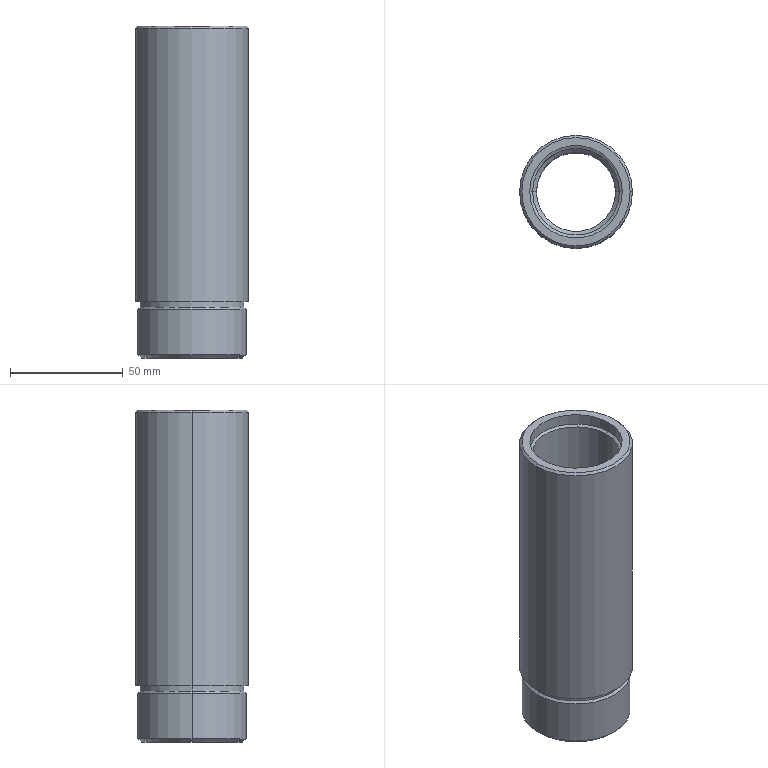Part | SolidWorks | features Chamfer 4, RevCut 2, Extrusion 1, ICE 1 | 1 solid | 25 faces | box 50 x 50 x 147 mm | volume 134333 mm3 | cylinder 12 | cone 10 | plane 3 | commonest cylinder face diameters 35 x2 38.5 x2 41 x2 46 x2 48 x2 50 x2
STEP:
#1=CARTESIAN_POINT('',(-17.5,0.,109.));
#2=VERTEX_POINT('',#1);
#3=CARTESIAN_POINT('',(17.5,0.,109.));
#4=VERTEX_POINT('',#3);
#5=CARTESIAN_POINT('',(0.,0.,109.));
#6=DIRECTION('',(0.,0.,1.));
#7=DIRECTION('',(1.,0.,0.));
#8=AXIS2_PLACEMENT_3D('',#5,#6,#7);
#9=CIRCLE('',#8,17.5);
#10=EDGE_CURVE('',#2,#4,#9,.T.);
#11=ORIENTED_EDGE('',*,*,#10,.F.);
#12=CARTESIAN_POINT('',(-19.25,0.,110.75));
#13=VERTEX_POINT('',#12);
#14=CARTESIAN_POINT('',(-19.25,0.,110.75));
#15=DIRECTION('',(-0.7071,0.,0.7071));
#16=VECTOR('',#15,1000.);
#17=LINE('',#14,#16);
#18=EDGE_CURVE('',#2,#13,#17,.T.);
#19=ORIENTED_EDGE('',*,*,#18,.T.);
#20=CARTESIAN_POINT('',(19.25,0.,110.75));
#21=VERTEX_POINT('',#20);
#22=CARTESIAN_POINT('',(0.,0.,110.75));
#23=DIRECTION('',(0.,0.,-1.));
#24=DIRECTION('',(1.,0.,0.));
#25=AXIS2_PLACEMENT_3D('',#22,#23,#24);
#26=CIRCLE('',#25,19.25);
#27=EDGE_CURVE('',#21,#13,#26,.T.);
#28=ORIENTED_EDGE('',*,*,#27,.F.);
#29=CARTESIAN_POINT('',(19.25,0.,110.75));
#30=DIRECTION('',(0.7071,0.,0.7071));
#31=VECTOR('',#30,1000.);
#32=LINE('',#29,#31);
#33=EDGE_CURVE('',#4,#21,#32,.T.);
#34=ORIENTED_EDGE('',*,*,#33,.F.);
#35=EDGE_LOOP('',(#11,#19,#28,#34));
#36=FACE_OUTER_BOUND('',#35,.T.);
#37=CARTESIAN_POINT('',(0.,0.,110.75));
#38=DIRECTION('',(0.,0.,1.));
#39=DIRECTION('',(1.,0.,0.));
#40=AXIS2_PLACEMENT_3D('',#37,#38,#39);
#41=CONICAL_SURFACE('',#40,19.25,0.7854);
#42=ADVANCED_FACE('',(#36),#41,.F.);
#43=CARTESIAN_POINT('',(19.25,0.,141.278));
#44=VERTEX_POINT('',#43);
#45=CARTESIAN_POINT('',(-19.25,0.,141.278));
#46=VERTEX_POINT('',#45);
#47=CARTESIAN_POINT('',(0.,0.,141.278));
#48=DIRECTION('',(0.,0.,-1.));
#49=DIRECTION('',(-1.,0.,0.));
#50=AXIS2_PLACEMENT_3D('',#47,#48,#49);
#51=CIRCLE('',#50,19.25);
#52=EDGE_CURVE('',#44,#46,#51,.T.);
#53=ORIENTED_EDGE('',*,*,#52,.F.);
#54=CARTESIAN_POINT('',(19.25,0.,0.));
#55=DIRECTION('',(0.,0.,-1.));
#56=VECTOR('',#55,1000.);
#57=LINE('',#54,#56);
#58=EDGE_CURVE('',#44,#21,#57,.T.);
#59=ORIENTED_EDGE('',*,*,#58,.T.);
#60=ORIENTED_EDGE('',*,*,#27,.T.);
#61=CARTESIAN_POINT('',(-19.25,0.,0.));
#62=DIRECTION('',(0.,0.,-1.));
#63=VECTOR('',#62,1000.);
#64=LINE('',#61,#63);
#65=EDGE_CURVE('',#46,#13,#64,.T.);
#66=ORIENTED_EDGE('',*,*,#65,.F.);
#67=EDGE_LOOP('',(#53,#59,#60,#66));
#68=FACE_OUTER_BOUND('',#67,.T.);
#69=CARTESIAN_POINT('',(0.,0.,0.));
#70=DIRECTION('',(0.,0.,-1.));
#71=DIRECTION('',(-1.,0.,0.));
#72=AXIS2_PLACEMENT_3D('',#69,#70,#71);
#73=CYLINDRICAL_SURFACE('',#72,19.25);
#74=ADVANCED_FACE('',(#68),#73,.F.);
#75=ORIENTED_EDGE('',*,*,#52,.T.);
#76=CARTESIAN_POINT('',(-20.5,0.,142.));
#77=VERTEX_POINT('',#76);
#78=CARTESIAN_POINT('',(-20.5,0.,142.));
#79=DIRECTION('',(-0.866,0.,0.5));
#80=VECTOR('',#79,1000.);
#81=LINE('',#78,#80);
#82=EDGE_CURVE('',#46,#77,#81,.T.);
#83=ORIENTED_EDGE('',*,*,#82,.T.);
#84=CARTESIAN_POINT('',(20.5,0.,142.));
#85=VERTEX_POINT('',#84);
#86=CARTESIAN_POINT('',(0.,0.,142.));
#87=DIRECTION('',(0.,0.,-1.));
#88=DIRECTION('',(-1.,0.,0.));
#89=AXIS2_PLACEMENT_3D('',#86,#87,#88);
#90=CIRCLE('',#89,20.5);
#91=EDGE_CURVE('',#85,#77,#90,.T.);
#92=ORIENTED_EDGE('',*,*,#91,.F.);
#93=CARTESIAN_POINT('',(20.5,0.,142.));
#94=DIRECTION('',(0.866,0.,0.5));
#95=VECTOR('',#94,1000.);
#96=LINE('',#93,#95);
#97=EDGE_CURVE('',#44,#85,#96,.T.);
#98=ORIENTED_EDGE('',*,*,#97,.F.);
#99=EDGE_LOOP('',(#75,#83,#92,#98));
#100=FACE_OUTER_BOUND('',#99,.T.);
#101=CARTESIAN_POINT('',(0.,0.,142.));
#102=DIRECTION('',(0.,0.,1.));
#103=DIRECTION('',(1.,0.,0.));
#104=AXIS2_PLACEMENT_3D('',#101,#102,#103);
#105=CONICAL_SURFACE('',#104,20.5,1.047);
#106=ADVANCED_FACE('',(#100),#105,.F.);
#107=CARTESIAN_POINT('',(20.5,0.,147.));
#108=VERTEX_POINT('',#107);
#109=CARTESIAN_POINT('',(-20.5,0.,147.));
#110=VERTEX_POINT('',#109);
#111=CARTESIAN_POINT('',(0.,0.,147.));
#112=DIRECTION('',(0.,0.,-1.));
#113=DIRECTION('',(-1.,0.,0.));
#114=AXIS2_PLACEMENT_3D('',#111,#112,#113);
#115=CIRCLE('',#114,20.5);
#116=EDGE_CURVE('',#108,#110,#115,.T.);
#117=ORIENTED_EDGE('',*,*,#116,.F.);
#118=CARTESIAN_POINT('',(20.5,0.,0.));
#119=DIRECTION('',(0.,0.,-1.));
#120=VECTOR('',#119,1000.);
#121=LINE('',#118,#120);
#122=EDGE_CURVE('',#108,#85,#121,.T.);
#123=ORIENTED_EDGE('',*,*,#122,.T.);
#124=ORIENTED_EDGE('',*,*,#91,.T.);
#125=CARTESIAN_POINT('',(-20.5,0.,0.));
#126=DIRECTION('',(0.,0.,-1.));
#127=VECTOR('',#126,1000.);
#128=LINE('',#125,#127);
#129=EDGE_CURVE('',#110,#77,#128,.T.);
#130=ORIENTED_EDGE('',*,*,#129,.F.);
#131=EDGE_LOOP('',(#117,#123,#124,#130));
#132=FACE_OUTER_BOUND('',#131,.T.);
#133=CARTESIAN_POINT('',(0.,0.,0.));
#134=DIRECTION('',(0.,0.,-1.));
#135=DIRECTION('',(-1.,0.,0.));
#136=AXIS2_PLACEMENT_3D('',#133,#134,#135);
#137=CYLINDRICAL_SURFACE('',#136,20.5);
#138=ADVANCED_FACE('',(#132),#137,.F.);
#139=CARTESIAN_POINT('',(24.,0.,147.));
#140=VERTEX_POINT('',#139);
#141=CARTESIAN_POINT('',(-24.,0.,147.));
#142=VERTEX_POINT('',#141);
#143=CARTESIAN_POINT('',(0.,0.,147.));
#144=DIRECTION('',(0.,0.,1.));
#145=DIRECTION('',(1.,0.,0.));
#146=AXIS2_PLACEMENT_3D('',#143,#144,#145);
#147=CIRCLE('',#146,24.);
#148=EDGE_CURVE('',#140,#142,#147,.T.);
#149=ORIENTED_EDGE('',*,*,#148,.F.);
#150=CARTESIAN_POINT('',(25.,0.,146.));
#151=VERTEX_POINT('',#150);
#152=CARTESIAN_POINT('',(24.,0.,147.));
#153=DIRECTION('',(0.7071,0.,-0.7071));
#154=VECTOR('',#153,1000.);
#155=LINE('',#152,#154);
#156=EDGE_CURVE('',#140,#151,#155,.T.);
#157=ORIENTED_EDGE('',*,*,#156,.T.);
#158=CARTESIAN_POINT('',(-25.,0.,146.));
#159=VERTEX_POINT('',#158);
#160=CARTESIAN_POINT('',(0.,0.,146.));
#161=DIRECTION('',(0.,0.,-1.));
#162=DIRECTION('',(1.,0.,0.));
#163=AXIS2_PLACEMENT_3D('',#160,#161,#162);
#164=CIRCLE('',#163,25.);
#165=EDGE_CURVE('',#159,#151,#164,.T.);
#166=ORIENTED_EDGE('',*,*,#165,.F.);
#167=CARTESIAN_POINT('',(-24.,0.,147.));
#168=DIRECTION('',(-0.7071,0.,-0.7071));
#169=VECTOR('',#168,1000.);
#170=LINE('',#167,#169);
#171=EDGE_CURVE('',#142,#159,#170,.T.);
#172=ORIENTED_EDGE('',*,*,#171,.F.);
#173=EDGE_LOOP('',(#149,#157,#166,#172));
#174=FACE_OUTER_BOUND('',#173,.T.);
#175=CARTESIAN_POINT('',(0.,0.,147.));
#176=DIRECTION('',(0.,0.,-1.));
#177=DIRECTION('',(-1.,0.,0.));
#178=AXIS2_PLACEMENT_3D('',#175,#176,#177);
#179=CONICAL_SURFACE('',#178,24.,0.7854);
#180=ADVANCED_FACE('',(#174),#179,.T.);
#181=CARTESIAN_POINT('',(-22.5,0.,0.));
#182=VERTEX_POINT('',#181);
#183=CARTESIAN_POINT('',(22.5,0.,0.));
#184=VERTEX_POINT('',#183);
#185=CARTESIAN_POINT('',(0.,0.,0.));
#186=DIRECTION('',(0.,0.,-1.));
#187=DIRECTION('',(1.,0.,0.));
#188=AXIS2_PLACEMENT_3D('',#185,#186,#187);
#189=CIRCLE('',#188,22.5);
#190=EDGE_CURVE('',#182,#184,#189,.T.);
#191=ORIENTED_EDGE('',*,*,#190,.F.);
#192=CARTESIAN_POINT('',(-24.,0.,1.5));
#193=VERTEX_POINT('',#192);
#194=CARTESIAN_POINT('',(-22.5,0.,0.));
#195=DIRECTION('',(-0.7071,0.,0.7071));
#196=VECTOR('',#195,1000.);
#197=LINE('',#194,#196);
#198=EDGE_CURVE('',#182,#193,#197,.T.);
#199=ORIENTED_EDGE('',*,*,#198,.T.);
#200=CARTESIAN_POINT('',(24.,0.,1.5));
#201=VERTEX_POINT('',#200);
#202=CARTESIAN_POINT('',(0.,0.,1.5));
#203=DIRECTION('',(0.,0.,1.));
#204=DIRECTION('',(1.,0.,0.));
#205=AXIS2_PLACEMENT_3D('',#202,#203,#204);
#206=CIRCLE('',#205,24.);
#207=EDGE_CURVE('',#201,#193,#206,.T.);
#208=ORIENTED_EDGE('',*,*,#207,.F.);
#209=CARTESIAN_POINT('',(22.5,0.,0.));
#210=DIRECTION('',(0.7071,0.,0.7071));
#211=VECTOR('',#210,1000.);
#212=LINE('',#209,#211);
#213=EDGE_CURVE('',#184,#201,#212,.T.);
#214=ORIENTED_EDGE('',*,*,#213,.F.);
#215=EDGE_LOOP('',(#191,#199,#208,#214));
#216=FACE_OUTER_BOUND('',#215,.T.);
#217=CARTESIAN_POINT('',(0.,0.,0.));
#218=DIRECTION('',(0.,0.,1.));
#219=DIRECTION('',(1.,0.,0.));
#220=AXIS2_PLACEMENT_3D('',#217,#218,#219);
#221=CONICAL_SURFACE('',#220,22.5,0.7854);
#222=ADVANCED_FACE('',(#216),#221,.T.);
#223=CARTESIAN_POINT('',(23.,0.,22.5));
#224=VERTEX_POINT('',#223);
#225=CARTESIAN_POINT('',(-23.,0.,22.5));
#226=VERTEX_POINT('',#225);
#227=CARTESIAN_POINT('',(0.,0.,22.5));
#228=DIRECTION('',(0.,0.,1.));
#229=DIRECTION('',(-1.,0.,0.));
#230=AXIS2_PLACEMENT_3D('',#227,#228,#229);
#231=CIRCLE('',#230,23.);
#232=EDGE_CURVE('',#224,#226,#231,.T.);
#233=ORIENTED_EDGE('',*,*,#232,.F.);
#234=CARTESIAN_POINT('',(24.,0.,21.5));
#235=VERTEX_POINT('',#234);
#236=CARTESIAN_POINT('',(24.,0.,21.5));
#237=DIRECTION('',(0.7071,0.,-0.7071));
#238=VECTOR('',#237,1000.);
#239=LINE('',#236,#238);
#240=EDGE_CURVE('',#224,#235,#239,.T.);
#241=ORIENTED_EDGE('',*,*,#240,.T.);
#242=CARTESIAN_POINT('',(-24.,0.,21.5));
#243=VERTEX_POINT('',#242);
#244=CARTESIAN_POINT('',(0.,0.,21.5));
#245=DIRECTION('',(0.,0.,-1.));
#246=DIRECTION('',(1.,0.,0.));
#247=AXIS2_PLACEMENT_3D('',#244,#245,#246);
#248=CIRCLE('',#247,24.);
#249=EDGE_CURVE('',#243,#235,#248,.T.);
#250=ORIENTED_EDGE('',*,*,#249,.F.);
#251=CARTESIAN_POINT('',(-24.,0.,21.5));
#252=DIRECTION('',(-0.7071,0.,-0.7071));
#253=VECTOR('',#252,1000.);
#254=LINE('',#251,#253);
#255=EDGE_CURVE('',#226,#243,#254,.T.);
#256=ORIENTED_EDGE('',*,*,#255,.F.);
#257=EDGE_LOOP('',(#233,#241,#250,#256));
#258=FACE_OUTER_BOUND('',#257,.T.);
#259=CARTESIAN_POINT('',(0.,0.,21.5));
#260=DIRECTION('',(0.,0.,-1.));
#261=DIRECTION('',(-1.,0.,0.));
#262=AXIS2_PLACEMENT_3D('',#259,#260,#261);
#263=CONICAL_SURFACE('',#262,24.,0.7854);
#264=ADVANCED_FACE('',(#258),#263,.T.);
#265=CARTESIAN_POINT('',(-23.,0.,25.));
#266=VERTEX_POINT('',#265);
#267=CARTESIAN_POINT('',(23.,0.,25.));
#268=VERTEX_POINT('',#267);
#269=CARTESIAN_POINT('',(0.,0.,25.));
#270=DIRECTION('',(0.,0.,-1.));
#271=DIRECTION('',(-1.,0.,0.));
#272=AXIS2_PLACEMENT_3D('',#269,#270,#271);
#273=CIRCLE('',#272,23.);
#274=EDGE_CURVE('',#266,#268,#273,.T.);
#275=ORIENTED_EDGE('',*,*,#274,.T.);
#276=CARTESIAN_POINT('',(23.,0.,0.));
#277=DIRECTION('',(0.,0.,-1.));
#278=VECTOR('',#277,1000.);
#279=LINE('',#276,#278);
#280=EDGE_CURVE('',#268,#224,#279,.T.);
#281=ORIENTED_EDGE('',*,*,#280,.T.);
#282=ORIENTED_EDGE('',*,*,#232,.T.);
#283=CARTESIAN_POINT('',(-23.,0.,0.));
#284=DIRECTION('',(0.,0.,-1.));
#285=VECTOR('',#284,1000.);
#286=LINE('',#283,#285);
#287=EDGE_CURVE('',#266,#226,#286,.T.);
#288=ORIENTED_EDGE('',*,*,#287,.F.);
#289=EDGE_LOOP('',(#275,#281,#282,#288));
#290=FACE_OUTER_BOUND('',#289,.T.);
#291=CARTESIAN_POINT('',(0.,0.,0.));
#292=DIRECTION('',(0.,0.,-1.));
#293=DIRECTION('',(-1.,0.,0.));
#294=AXIS2_PLACEMENT_3D('',#291,#292,#293);
#295=CYLINDRICAL_SURFACE('',#294,23.);
#296=ADVANCED_FACE('',(#290),#295,.T.);
#297=ORIENTED_EDGE('',*,*,#249,.T.);
#298=CARTESIAN_POINT('',(24.,0.,0.));
#299=DIRECTION('',(0.,0.,-1.));
#300=VECTOR('',#299,1000.);
#301=LINE('',#298,#300);
#302=EDGE_CURVE('',#235,#201,#301,.T.);
#303=ORIENTED_EDGE('',*,*,#302,.T.);
#304=ORIENTED_EDGE('',*,*,#207,.T.);
#305=CARTESIAN_POINT('',(-24.,0.,0.));
#306=DIRECTION('',(0.,0.,-1.));
#307=VECTOR('',#306,1000.);
#308=LINE('',#305,#307);
#309=EDGE_CURVE('',#243,#193,#308,.T.);
#310=ORIENTED_EDGE('',*,*,#309,.F.);
#311=EDGE_LOOP('',(#297,#303,#304,#310));
#312=FACE_OUTER_BOUND('',#311,.T.);
#313=CARTESIAN_POINT('',(0.,0.,0.));
#314=DIRECTION('',(0.,0.,-1.));
#315=DIRECTION('',(-1.,0.,0.));
#316=AXIS2_PLACEMENT_3D('',#313,#314,#315);
#317=CYLINDRICAL_SURFACE('',#316,24.);
#318=ADVANCED_FACE('',(#312),#317,.T.);
#319=ORIENTED_EDGE('',*,*,#165,.T.);
#320=CARTESIAN_POINT('',(25.,0.,25.));
#321=VERTEX_POINT('',#320);
#322=CARTESIAN_POINT('',(25.,0.,147.));
#323=DIRECTION('',(0.,0.,-1.));
#324=VECTOR('',#323,1000.);
#325=LINE('',#322,#324);
#326=EDGE_CURVE('',#151,#321,#325,.T.);
#327=ORIENTED_EDGE('',*,*,#326,.T.);
#328=CARTESIAN_POINT('',(-25.,0.,25.));
#329=VERTEX_POINT('',#328);
#330=CARTESIAN_POINT('',(0.,0.,25.));
#331=DIRECTION('',(0.,0.,-1.));
#332=DIRECTION('',(-1.,0.,0.));
#333=AXIS2_PLACEMENT_3D('',#330,#331,#332);
#334=CIRCLE('',#333,25.);
#335=EDGE_CURVE('',#329,#321,#334,.T.);
#336=ORIENTED_EDGE('',*,*,#335,.F.);
#337=CARTESIAN_POINT('',(-25.,0.,147.));
#338=DIRECTION('',(0.,0.,-1.));
#339=VECTOR('',#338,1000.);
#340=LINE('',#337,#339);
#341=EDGE_CURVE('',#159,#329,#340,.T.);
#342=ORIENTED_EDGE('',*,*,#341,.F.);
#343=EDGE_LOOP('',(#319,#327,#336,#342));
#344=FACE_OUTER_BOUND('',#343,.T.);
#345=CARTESIAN_POINT('',(0.,0.,147.));
#346=DIRECTION('',(0.,0.,-1.));
#347=DIRECTION('',(-1.,0.,0.));
#348=AXIS2_PLACEMENT_3D('',#345,#346,#347);
#349=CYLINDRICAL_SURFACE('',#348,25.);
#350=ADVANCED_FACE('',(#344),#349,.T.);
#351=ORIENTED_EDGE('',*,*,#10,.T.);
#352=CARTESIAN_POINT('',(17.5,0.,0.));
#353=VERTEX_POINT('',#352);
#354=CARTESIAN_POINT('',(17.5,0.,147.));
#355=DIRECTION('',(0.,0.,-1.));
#356=VECTOR('',#355,1000.);
#357=LINE('',#354,#356);
#358=EDGE_CURVE('',#4,#353,#357,.T.);
#359=ORIENTED_EDGE('',*,*,#358,.T.);
#360=CARTESIAN_POINT('',(-17.5,0.,0.));
#361=VERTEX_POINT('',#360);
#362=CARTESIAN_POINT('',(0.,0.,0.));
#363=DIRECTION('',(0.,0.,1.));
#364=DIRECTION('',(1.,0.,0.));
#365=AXIS2_PLACEMENT_3D('',#362,#363,#364);
#366=CIRCLE('',#365,17.5);
#367=EDGE_CURVE('',#361,#353,#366,.T.);
#368=ORIENTED_EDGE('',*,*,#367,.F.);
#369=CARTESIAN_POINT('',(-17.5,0.,147.));
#370=DIRECTION('',(0.,0.,-1.));
#371=VECTOR('',#370,1000.);
#372=LINE('',#369,#371);
#373=EDGE_CURVE('',#2,#361,#372,.T.);
#374=ORIENTED_EDGE('',*,*,#373,.F.);
#375=EDGE_LOOP('',(#351,#359,#368,#374));
#376=FACE_OUTER_BOUND('',#375,.T.);
#377=CARTESIAN_POINT('',(0.,0.,147.));
#378=DIRECTION('',(0.,0.,-1.));
#379=DIRECTION('',(-1.,0.,0.));
#380=AXIS2_PLACEMENT_3D('',#377,#378,#379);
#381=CYLINDRICAL_SURFACE('',#380,17.5);
#382=ADVANCED_FACE('',(#376),#381,.F.);
#383=ORIENTED_EDGE('',*,*,#358,.F.);
#384=CARTESIAN_POINT('',(0.,0.,109.));
#385=DIRECTION('',(0.,0.,1.));
#386=DIRECTION('',(1.,0.,0.));
#387=AXIS2_PLACEMENT_3D('',#384,#385,#386);
#388=CIRCLE('',#387,17.5);
#389=EDGE_CURVE('',#4,#2,#388,.T.);
#390=ORIENTED_EDGE('',*,*,#389,.T.);
#391=ORIENTED_EDGE('',*,*,#373,.T.);
#392=CARTESIAN_POINT('',(0.,0.,0.));
#393=DIRECTION('',(0.,0.,1.));
#394=DIRECTION('',(1.,0.,0.));
#395=AXIS2_PLACEMENT_3D('',#392,#393,#394);
#396=CIRCLE('',#395,17.5);
#397=EDGE_CURVE('',#353,#361,#396,.T.);
#398=ORIENTED_EDGE('',*,*,#397,.F.);
#399=EDGE_LOOP('',(#383,#390,#391,#398));
#400=FACE_OUTER_BOUND('',#399,.T.);
#401=CARTESIAN_POINT('',(0.,0.,147.));
#402=DIRECTION('',(0.,0.,-1.));
#403=DIRECTION('',(-1.,0.,0.));
#404=AXIS2_PLACEMENT_3D('',#401,#402,#403);
#405=CYLINDRICAL_SURFACE('',#404,17.5);
#406=ADVANCED_FACE('',(#400),#405,.F.);
#407=CARTESIAN_POINT('',(0.,0.,0.));
#408=DIRECTION('',(0.,0.,-1.));
#409=DIRECTION('',(1.,0.,0.));
#410=AXIS2_PLACEMENT_3D('',#407,#408,#409);
#411=CIRCLE('',#410,22.5);
#412=EDGE_CURVE('',#184,#182,#411,.T.);
#413=ORIENTED_EDGE('',*,*,#412,.T.);
#414=ORIENTED_EDGE('',*,*,#190,.T.);
#415=EDGE_LOOP('',(#413,#414));
#416=FACE_OUTER_BOUND('',#415,.T.);
#417=ORIENTED_EDGE('',*,*,#367,.T.);
#418=ORIENTED_EDGE('',*,*,#397,.T.);
#419=EDGE_LOOP('',(#417,#418));
#420=FACE_BOUND('',#419,.T.);
#421=CARTESIAN_POINT('',(0.,0.,0.));
#422=DIRECTION('',(0.,0.,1.));
#423=DIRECTION('',(1.,0.,0.));
#424=AXIS2_PLACEMENT_3D('',#421,#422,#423);
#425=PLANE('',#424);
#426=ADVANCED_FACE('',(#416,#420),#425,.F.);
#427=ORIENTED_EDGE('',*,*,#326,.F.);
#428=CARTESIAN_POINT('',(0.,0.,146.));
#429=DIRECTION('',(0.,0.,-1.));
#430=DIRECTION('',(1.,0.,0.));
#431=AXIS2_PLACEMENT_3D('',#428,#429,#430);
#432=CIRCLE('',#431,25.);
#433=EDGE_CURVE('',#151,#159,#432,.T.);
#434=ORIENTED_EDGE('',*,*,#433,.T.);
#435=ORIENTED_EDGE('',*,*,#341,.T.);
#436=CARTESIAN_POINT('',(0.,0.,25.));
#437=DIRECTION('',(0.,0.,-1.));
#438=DIRECTION('',(-1.,0.,0.));
#439=AXIS2_PLACEMENT_3D('',#436,#437,#438);
#440=CIRCLE('',#439,25.);
#441=EDGE_CURVE('',#321,#329,#440,.T.);
#442=ORIENTED_EDGE('',*,*,#441,.F.);
#443=EDGE_LOOP('',(#427,#434,#435,#442));
#444=FACE_OUTER_BOUND('',#443,.T.);
#445=CARTESIAN_POINT('',(0.,0.,147.));
#446=DIRECTION('',(0.,0.,-1.));
#447=DIRECTION('',(-1.,0.,0.));
#448=AXIS2_PLACEMENT_3D('',#445,#446,#447);
#449=CYLINDRICAL_SURFACE('',#448,25.);
#450=ADVANCED_FACE('',(#444),#449,.T.);
#451=CARTESIAN_POINT('',(0.,0.,147.));
#452=DIRECTION('',(0.,0.,-1.));
#453=DIRECTION('',(-1.,0.,0.));
#454=AXIS2_PLACEMENT_3D('',#451,#452,#453);
#455=CIRCLE('',#454,20.5);
#456=EDGE_CURVE('',#110,#108,#455,.T.);
#457=ORIENTED_EDGE('',*,*,#456,.T.);
#458=ORIENTED_EDGE('',*,*,#116,.T.);
#459=EDGE_LOOP('',(#457,#458));
#460=FACE_BOUND('',#459,.T.);
#461=CARTESIAN_POINT('',(0.,0.,147.));
#462=DIRECTION('',(0.,0.,1.));
#463=DIRECTION('',(1.,0.,0.));
#464=AXIS2_PLACEMENT_3D('',#461,#462,#463);
#465=CIRCLE('',#464,24.);
#466=EDGE_CURVE('',#142,#140,#465,.T.);
#467=ORIENTED_EDGE('',*,*,#466,.T.);
#468=ORIENTED_EDGE('',*,*,#148,.T.);
#469=EDGE_LOOP('',(#467,#468));
#470=FACE_OUTER_BOUND('',#469,.T.);
#471=CARTESIAN_POINT('',(0.,0.,147.));
#472=DIRECTION('',(0.,0.,1.));
#473=DIRECTION('',(1.,0.,0.));
#474=AXIS2_PLACEMENT_3D('',#471,#472,#473);
#475=PLANE('',#474);
#476=ADVANCED_FACE('',(#460,#470),#475,.T.);
#477=ORIENTED_EDGE('',*,*,#302,.F.);
#478=CARTESIAN_POINT('',(0.,0.,21.5));
#479=DIRECTION('',(0.,0.,-1.));
#480=DIRECTION('',(1.,0.,0.));
#481=AXIS2_PLACEMENT_3D('',#478,#479,#480);
#482=CIRCLE('',#481,24.);
#483=EDGE_CURVE('',#235,#243,#482,.T.);
#484=ORIENTED_EDGE('',*,*,#483,.T.);
#485=ORIENTED_EDGE('',*,*,#309,.T.);
#486=CARTESIAN_POINT('',(0.,0.,1.5));
#487=DIRECTION('',(0.,0.,1.));
#488=DIRECTION('',(1.,0.,0.));
#489=AXIS2_PLACEMENT_3D('',#486,#487,#488);
#490=CIRCLE('',#489,24.);
#491=EDGE_CURVE('',#193,#201,#490,.T.);
#492=ORIENTED_EDGE('',*,*,#491,.T.);
#493=EDGE_LOOP('',(#477,#484,#485,#492));
#494=FACE_OUTER_BOUND('',#493,.T.);
#495=CARTESIAN_POINT('',(0.,0.,0.));
#496=DIRECTION('',(0.,0.,-1.));
#497=DIRECTION('',(-1.,0.,0.));
#498=AXIS2_PLACEMENT_3D('',#495,#496,#497);
#499=CYLINDRICAL_SURFACE('',#498,24.);
#500=ADVANCED_FACE('',(#494),#499,.T.);
#501=ORIENTED_EDGE('',*,*,#280,.F.);
#502=CARTESIAN_POINT('',(0.,0.,25.));
#503=DIRECTION('',(0.,0.,-1.));
#504=DIRECTION('',(-1.,0.,0.));
#505=AXIS2_PLACEMENT_3D('',#502,#503,#504);
#506=CIRCLE('',#505,23.);
#507=EDGE_CURVE('',#268,#266,#506,.T.);
#508=ORIENTED_EDGE('',*,*,#507,.T.);
#509=ORIENTED_EDGE('',*,*,#287,.T.);
#510=CARTESIAN_POINT('',(0.,0.,22.5));
#511=DIRECTION('',(0.,0.,1.));
#512=DIRECTION('',(-1.,0.,0.));
#513=AXIS2_PLACEMENT_3D('',#510,#511,#512);
#514=CIRCLE('',#513,23.);
#515=EDGE_CURVE('',#226,#224,#514,.T.);
#516=ORIENTED_EDGE('',*,*,#515,.T.);
#517=EDGE_LOOP('',(#501,#508,#509,#516));
#518=FACE_OUTER_BOUND('',#517,.T.);
#519=CARTESIAN_POINT('',(0.,0.,0.));
#520=DIRECTION('',(0.,0.,-1.));
#521=DIRECTION('',(-1.,0.,0.));
#522=AXIS2_PLACEMENT_3D('',#519,#520,#521);
#523=CYLINDRICAL_SURFACE('',#522,23.);
#524=ADVANCED_FACE('',(#518),#523,.T.);
#525=ORIENTED_EDGE('',*,*,#335,.T.);
#526=ORIENTED_EDGE('',*,*,#441,.T.);
#527=EDGE_LOOP('',(#525,#526));
#528=FACE_OUTER_BOUND('',#527,.T.);
#529=ORIENTED_EDGE('',*,*,#274,.F.);
#530=ORIENTED_EDGE('',*,*,#507,.F.);
#531=EDGE_LOOP('',(#529,#530));
#532=FACE_BOUND('',#531,.T.);
#533=CARTESIAN_POINT('',(23.,0.,25.));
#534=DIRECTION('',(0.,0.,-1.));
#535=DIRECTION('',(-1.,0.,0.));
#536=AXIS2_PLACEMENT_3D('',#533,#534,#535);
#537=PLANE('',#536);
#538=ADVANCED_FACE('',(#528,#532),#537,.T.);
#539=ORIENTED_EDGE('',*,*,#240,.F.);
#540=ORIENTED_EDGE('',*,*,#515,.F.);
#541=ORIENTED_EDGE('',*,*,#255,.T.);
#542=ORIENTED_EDGE('',*,*,#483,.F.);
#543=EDGE_LOOP('',(#539,#540,#541,#542));
#544=FACE_OUTER_BOUND('',#543,.T.);
#545=CARTESIAN_POINT('',(0.,0.,21.5));
#546=DIRECTION('',(0.,0.,-1.));
#547=DIRECTION('',(-1.,0.,0.));
#548=AXIS2_PLACEMENT_3D('',#545,#546,#547);
#549=CONICAL_SURFACE('',#548,24.,0.7854);
#550=ADVANCED_FACE('',(#544),#549,.T.);
#551=ORIENTED_EDGE('',*,*,#198,.F.);
#552=ORIENTED_EDGE('',*,*,#412,.F.);
#553=ORIENTED_EDGE('',*,*,#213,.T.);
#554=ORIENTED_EDGE('',*,*,#491,.F.);
#555=EDGE_LOOP('',(#551,#552,#553,#554));
#556=FACE_OUTER_BOUND('',#555,.T.);
#557=CARTESIAN_POINT('',(0.,0.,0.));
#558=DIRECTION('',(0.,0.,1.));
#559=DIRECTION('',(1.,0.,0.));
#560=AXIS2_PLACEMENT_3D('',#557,#558,#559);
#561=CONICAL_SURFACE('',#560,22.5,0.7854);
#562=ADVANCED_FACE('',(#556),#561,.T.);
#563=ORIENTED_EDGE('',*,*,#156,.F.);
#564=ORIENTED_EDGE('',*,*,#466,.F.);
#565=ORIENTED_EDGE('',*,*,#171,.T.);
#566=ORIENTED_EDGE('',*,*,#433,.F.);
#567=EDGE_LOOP('',(#563,#564,#565,#566));
#568=FACE_OUTER_BOUND('',#567,.T.);
#569=CARTESIAN_POINT('',(0.,0.,147.));
#570=DIRECTION('',(0.,0.,-1.));
#571=DIRECTION('',(-1.,0.,0.));
#572=AXIS2_PLACEMENT_3D('',#569,#570,#571);
#573=CONICAL_SURFACE('',#572,24.,0.7854);
#574=ADVANCED_FACE('',(#568),#573,.T.);
#575=ORIENTED_EDGE('',*,*,#122,.F.);
#576=ORIENTED_EDGE('',*,*,#456,.F.);
#577=ORIENTED_EDGE('',*,*,#129,.T.);
#578=CARTESIAN_POINT('',(0.,0.,142.));
#579=DIRECTION('',(0.,0.,-1.));
#580=DIRECTION('',(-1.,0.,0.));
#581=AXIS2_PLACEMENT_3D('',#578,#579,#580);
#582=CIRCLE('',#581,20.5);
#583=EDGE_CURVE('',#77,#85,#582,.T.);
#584=ORIENTED_EDGE('',*,*,#583,.T.);
#585=EDGE_LOOP('',(#575,#576,#577,#584));
#586=FACE_OUTER_BOUND('',#585,.T.);
#587=CARTESIAN_POINT('',(0.,0.,0.));
#588=DIRECTION('',(0.,0.,-1.));
#589=DIRECTION('',(-1.,0.,0.));
#590=AXIS2_PLACEMENT_3D('',#587,#588,#589);
#591=CYLINDRICAL_SURFACE('',#590,20.5);
#592=ADVANCED_FACE('',(#586),#591,.F.);
#593=ORIENTED_EDGE('',*,*,#82,.F.);
#594=CARTESIAN_POINT('',(0.,0.,141.278));
#595=DIRECTION('',(0.,0.,-1.));
#596=DIRECTION('',(-1.,0.,0.));
#597=AXIS2_PLACEMENT_3D('',#594,#595,#596);
#598=CIRCLE('',#597,19.25);
#599=EDGE_CURVE('',#46,#44,#598,.T.);
#600=ORIENTED_EDGE('',*,*,#599,.T.);
#601=ORIENTED_EDGE('',*,*,#97,.T.);
#602=ORIENTED_EDGE('',*,*,#583,.F.);
#603=EDGE_LOOP('',(#593,#600,#601,#602));
#604=FACE_OUTER_BOUND('',#603,.T.);
#605=CARTESIAN_POINT('',(0.,0.,142.));
#606=DIRECTION('',(0.,0.,1.));
#607=DIRECTION('',(1.,0.,0.));
#608=AXIS2_PLACEMENT_3D('',#605,#606,#607);
#609=CONICAL_SURFACE('',#608,20.5,1.047);
#610=ADVANCED_FACE('',(#604),#609,.F.);
#611=ORIENTED_EDGE('',*,*,#58,.F.);
#612=ORIENTED_EDGE('',*,*,#599,.F.);
#613=ORIENTED_EDGE('',*,*,#65,.T.);
#614=CARTESIAN_POINT('',(0.,0.,110.75));
#615=DIRECTION('',(0.,0.,-1.));
#616=DIRECTION('',(1.,0.,0.));
#617=AXIS2_PLACEMENT_3D('',#614,#615,#616);
#618=CIRCLE('',#617,19.25);
#619=EDGE_CURVE('',#13,#21,#618,.T.);
#620=ORIENTED_EDGE('',*,*,#619,.T.);
#621=EDGE_LOOP('',(#611,#612,#613,#620));
#622=FACE_OUTER_BOUND('',#621,.T.);
#623=CARTESIAN_POINT('',(0.,0.,0.));
#624=DIRECTION('',(0.,0.,-1.));
#625=DIRECTION('',(-1.,0.,0.));
#626=AXIS2_PLACEMENT_3D('',#623,#624,#625);
#627=CYLINDRICAL_SURFACE('',#626,19.25);
#628=ADVANCED_FACE('',(#622),#627,.F.);
#629=ORIENTED_EDGE('',*,*,#18,.F.);
#630=ORIENTED_EDGE('',*,*,#389,.F.);
#631=ORIENTED_EDGE('',*,*,#33,.T.);
#632=ORIENTED_EDGE('',*,*,#619,.F.);
#633=EDGE_LOOP('',(#629,#630,#631,#632));
#634=FACE_OUTER_BOUND('',#633,.T.);
#635=CARTESIAN_POINT('',(0.,0.,110.75));
#636=DIRECTION('',(0.,0.,1.));
#637=DIRECTION('',(1.,0.,0.));
#638=AXIS2_PLACEMENT_3D('',#635,#636,#637);
#639=CONICAL_SURFACE('',#638,19.25,0.7854);
#640=ADVANCED_FACE('',(#634),#639,.F.);
#641=CLOSED_SHELL('',(#42,#74,#106,#138,#180,#222,#264,#296,#318,#350,#382,#406,#426,#450,#476,#500,#524,#538,#550,#562,#574,#592,#610,#628,#640));
#642=MANIFOLD_SOLID_BREP('',#641);
#643=CARTESIAN_POINT('',(0.,0.,0.));
#644=DIRECTION('',(0.,0.,1.));
#645=DIRECTION('',(1.,0.,0.));
#646=AXIS2_PLACEMENT_3D('',#643,#644,#645);
#647=(LENGTH_UNIT()NAMED_UNIT(*)SI_UNIT(.MILLI.,.METRE.));
#648=UNCERTAINTY_MEASURE_WITH_UNIT(LENGTH_MEASURE(0.00001),#647,'','');
#649=(NAMED_UNIT(*)PLANE_ANGLE_UNIT()SI_UNIT($,.RADIAN.));
#650=(NAMED_UNIT(*)SI_UNIT($,.STERADIAN.)SOLID_ANGLE_UNIT());
#651=(GEOMETRIC_REPRESENTATION_CONTEXT(3)GLOBAL_UNCERTAINTY_ASSIGNED_CONTEXT((#648))GLOBAL_UNIT_ASSIGNED_CONTEXT((#647,#649,#650))REPRESENTATION_CONTEXT('',''));
#652=ADVANCED_BREP_SHAPE_REPRESENTATION('',(#642,#646),#651);